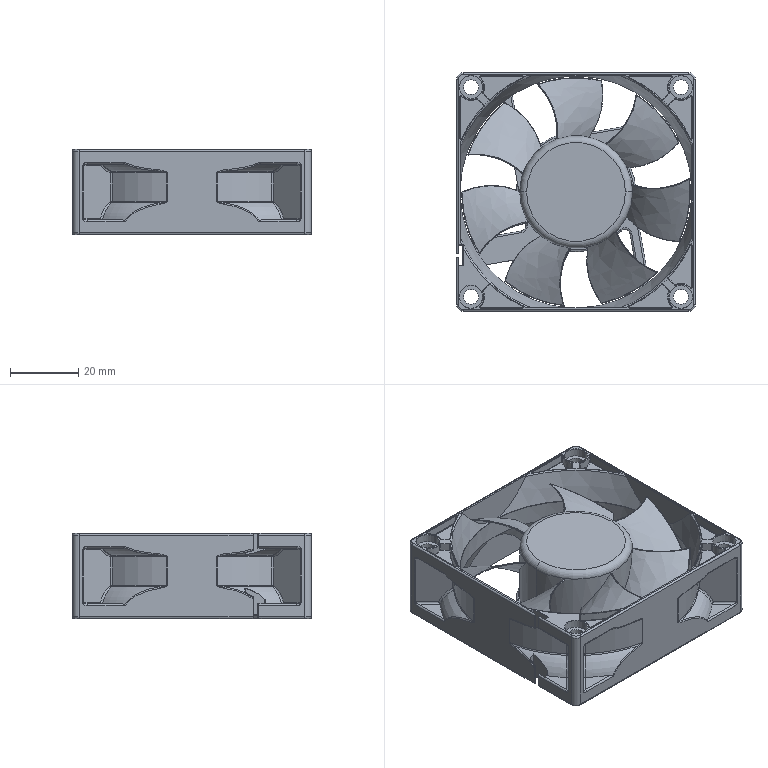Part | SolidWorks | features ICE 10, Fillet 8, CirPattern 2, MirrorPattern 2, CombineBodies 1, Extrusion 1, Helix 1, RevCut 1, Sweep 1 | 1 solid | 933 faces | box 70 x 70 x 25 mm | volume 39371 mm3 | cylinder 292 | torus 236 | spline 178 | plane 154 | sphere 56 | cone 17 | commonest cylinder face diameters 1 x75 0.6 x70 0.2 x60 7.7 x18 6.7 x16 73.848 x14